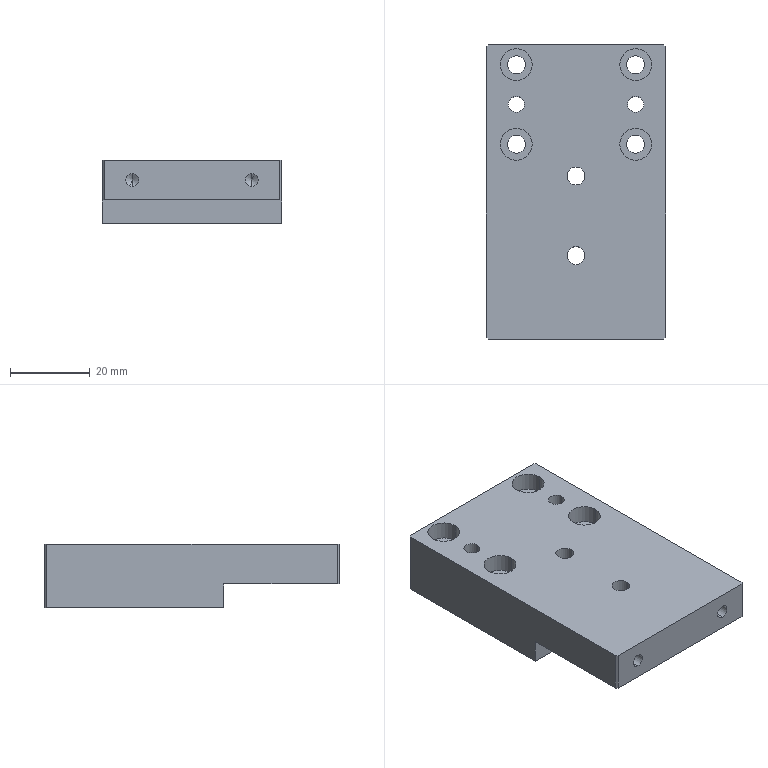Part | STEP file | 2082 Bag feed connecting plate A | 1 solid | 54 faces | box 45 x 74 x 16 mm | volume 42322 mm3 | cylinder 32 | plane 18 | cone 4 | commonest cylinder face diameters 4.5 x12 8 x12 3.3 x4 4 x4